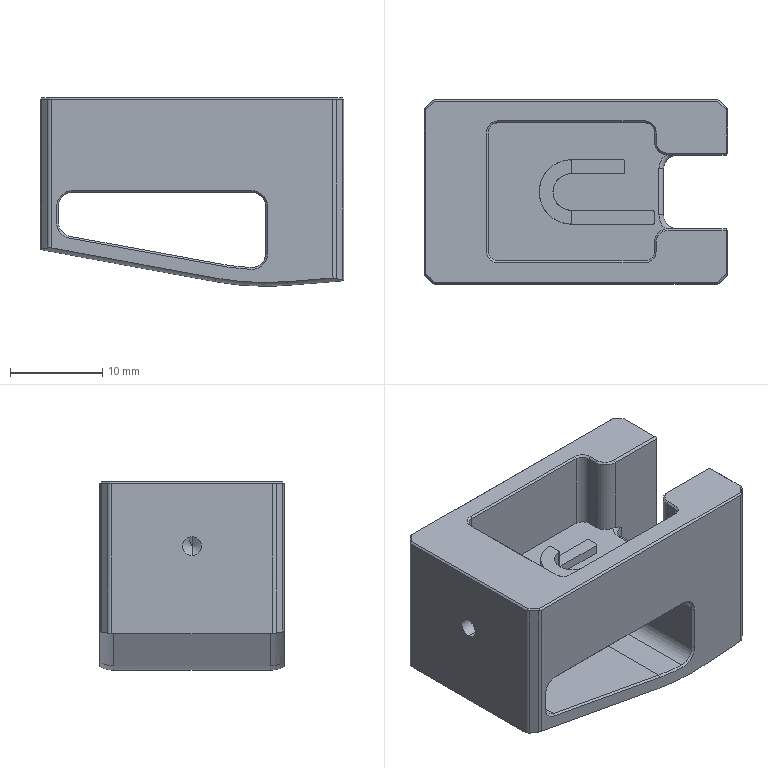NC program | NX | posted with a generic post | part box 33 x 20 x 20.478 mm
Lines 1201 to 2151 of 3438:
(PLANAR_MILL_COPY_1 , TOOL : D3)
N2394 T16 M6
N2396 G54
N2398 G17 G0 G90 X-16.129 Y-4.355 B0. C0. S9500 M3
N2400 G43 Z30. H16
N2402 Z-0.2
N2404 G94 G1 X-16.252 Y-4.41 F1000.
N2406 G3 X-16.838 Y-5.22 R1.
N2408 X-16.939 Y-6.5 R26.5
N2410 G1 X-15.658
N2412 G3 X-14.792 Y-6. R1.
N2414 G1 X-14.734 Y-5.9
N2416 G0 X-16.129 Y-4.355 Z-0.4
N2418 G1 X-16.252 Y-4.41
N2420 G3 X-16.838 Y-5.22 R1.
N2422 X-16.939 Y-6.5 R26.5
N2424 G1 X-15.658
N2426 G3 X-14.792 Y-6. R1.
N2428 G1 X-14.734 Y-5.9
N2430 G0 X-16.129 Y-4.355 Z-0.6
N2432 G1 X-16.252 Y-4.41
N2434 G3 X-16.838 Y-5.22 R1.
N2436 X-16.939 Y-6.5 R26.5
N2438 G1 X-15.658
N2440 G3 X-14.792 Y-6. R1.
N2442 G1 X-14.734 Y-5.9
N2444 G0 X-16.129 Y-4.355 Z-0.8
N2446 G1 X-16.252 Y-4.41
N2448 G3 X-16.838 Y-5.22 R1.
N2450 X-16.939 Y-6.5 R26.5
N2452 G1 X-15.658
N2454 G3 X-14.792 Y-6. R1.
N2456 G1 X-14.734 Y-5.9
N2458 G0 X-16.129 Y-4.355 Z-1.
N2460 G1 X-16.252 Y-4.41
N2462 G3 X-16.838 Y-5.22 R1.
N2464 X-16.939 Y-6.5 R26.5
N2466 G1 X-15.658
N2468 G3 X-14.792 Y-6. R1.
N2470 G1 X-14.734 Y-5.9
N2472 G0 X-16.129 Y-4.355 Z-1.2
N2474 G1 X-16.252 Y-4.41
N2476 G3 X-16.838 Y-5.22 R1.
N2478 X-16.939 Y-6.5 R26.5
N2480 G1 X-15.658
N2482 G3 X-14.792 Y-6. R1.
N2484 G1 X-14.734 Y-5.9
N2486 G0 X-16.129 Y-4.355 Z-1.4
N2488 G1 X-16.252 Y-4.41
N2490 G3 X-16.838 Y-5.22 R1.
N2492 X-16.939 Y-6.5 R26.5
N2494 G1 X-15.658
N2496 G3 X-14.792 Y-6. R1.
N2498 G1 X-14.734 Y-5.9
N2500 G0 X-16.129 Y-4.355 Z-1.6
N2502 G1 X-16.252 Y-4.41
N2504 G3 X-16.838 Y-5.22 R1.
N2506 X-16.939 Y-6.5 R26.5
N2508 G1 X-15.658
N2510 G3 X-14.792 Y-6. R1.
N2512 G1 X-14.734 Y-5.9
N2514 G0 X-16.129 Y-4.355 Z-1.8
N2516 G1 X-16.252 Y-4.41
N2518 G3 X-16.838 Y-5.22 R1.
N2520 X-16.939 Y-6.5 R26.5
N2522 G1 X-15.658
N2524 G3 X-14.792 Y-6. R1.
N2526 G1 X-14.734 Y-5.9
N2528 G0 X-16.129 Y-4.355 Z-2.
N2530 G1 X-16.252 Y-4.41
N2532 G3 X-16.838 Y-5.22 R1.
N2534 X-16.939 Y-6.5 R26.5
N2536 G1 X-15.658
N2538 G3 X-14.792 Y-6. R1.
N2540 G1 X-14.734 Y-5.9
N2542 G0 X-16.129 Y-4.355 Z-2.2
N2544 G1 X-16.252 Y-4.41
N2546 G3 X-16.838 Y-5.22 R1.
N2548 X-16.939 Y-6.5 R26.5
N2550 G1 X-15.658
N2552 G3 X-14.792 Y-6. R1.
N2554 G1 X-14.734 Y-5.9
N2556 G0 X-16.129 Y-4.355 Z-2.4
N2558 G1 X-16.252 Y-4.41
N2560 G3 X-16.838 Y-5.22 R1.
N2562 X-16.939 Y-6.5 R26.5
N2564 G1 X-15.658
N2566 G3 X-14.792 Y-6. R1.
N2568 G1 X-14.734 Y-5.9
N2570 G0 X-16.129 Y-4.355 Z-2.6
N2572 G1 X-16.252 Y-4.41
N2574 G3 X-16.838 Y-5.22 R1.
N2576 X-16.939 Y-6.5 R26.5
N2578 G1 X-15.658
N2580 G3 X-14.792 Y-6. R1.
N2582 G1 X-14.734 Y-5.9
N2584 G0 X-16.129 Y-4.355 Z-2.8
N2586 G1 X-16.252 Y-4.41
N2588 G3 X-16.838 Y-5.22 R1.
N2590 X-16.939 Y-6.5 R26.5
N2592 G1 X-15.658
N2594 G3 X-14.792 Y-6. R1.
N2596 G1 X-14.734 Y-5.9
N2598 G0 X-16.129 Y-4.355 Z-3.
N2600 G1 X-16.252 Y-4.41
N2602 G3 X-16.838 Y-5.22 R1.
N2604 X-16.939 Y-6.5 R26.5
N2606 G1 X-15.658
N2608 G3 X-14.792 Y-6. R1.
N2610 G1 X-14.734 Y-5.9
N2612 G0 X-16.129 Y-4.355 Z-3.2
N2614 G1 X-16.252 Y-4.41
N2616 G3 X-16.838 Y-5.22 R1.
N2618 X-16.939 Y-6.5 R26.5
N2620 G1 X-15.658
N2622 G3 X-14.792 Y-6. R1.
N2624 G1 X-14.734 Y-5.9
N2626 G0 X-16.129 Y-4.355 Z-3.4
N2628 G1 X-16.252 Y-4.41
N2630 G3 X-16.838 Y-5.22 R1.
N2632 X-16.939 Y-6.5 R26.5
N2634 G1 X-15.658
N2636 G3 X-14.792 Y-6. R1.
N2638 G1 X-14.734 Y-5.9
N2640 G0 X-16.129 Y-4.355 Z-3.6
N2642 G1 X-16.252 Y-4.41
N2644 G3 X-16.838 Y-5.22 R1.
N2646 X-16.939 Y-6.5 R26.5
N2648 G1 X-15.658
N2650 G3 X-14.792 Y-6. R1.
N2652 G1 X-14.734 Y-5.9
N2654 G0 X-16.129 Y-4.355 Z-3.8
N2656 G1 X-16.252 Y-4.41
N2658 G3 X-16.838 Y-5.22 R1.
N2660 X-16.939 Y-6.5 R26.5
N2662 G1 X-15.658
N2664 G3 X-14.792 Y-6. R1.
N2666 G1 X-14.734 Y-5.9
N2668 G0 X-16.129 Y-4.355 Z-4.
N2670 G1 X-16.252 Y-4.41
N2672 G3 X-16.838 Y-5.22 R1.
N2674 X-16.939 Y-6.5 R26.5
N2676 G1 X-15.658
N2678 G3 X-14.792 Y-6. R1.
N2680 G1 X-14.734 Y-5.9
N2682 G0 X-16.129 Y-4.355 Z-4.2
N2684 G1 X-16.252 Y-4.41
N2686 G3 X-16.838 Y-5.22 R1.
N2688 X-16.939 Y-6.5 R26.5
N2690 G1 X-15.658
N2692 G3 X-14.792 Y-6. R1.
N2694 G1 X-14.734 Y-5.9
N2696 G0 X-16.129 Y-4.355 Z-4.4
N2698 G1 X-16.252 Y-4.41
N2700 G3 X-16.838 Y-5.22 R1.
N2702 X-16.939 Y-6.5 R26.5
N2704 G1 X-15.658
N2706 G3 X-14.792 Y-6. R1.
N2708 G1 X-14.734 Y-5.9
N2710 G0 X-16.129 Y-4.355 Z-4.6
N2712 G1 X-16.252 Y-4.41
N2714 G3 X-16.838 Y-5.22 R1.
N2716 X-16.939 Y-6.5 R26.5
N2718 G1 X-15.658
N2720 G3 X-14.792 Y-6. R1.
N2722 G1 X-14.734 Y-5.9
N2724 G0 X-16.129 Y-4.355 Z-4.8
N2726 G1 X-16.252 Y-4.41
N2728 G3 X-16.838 Y-5.22 R1.
N2730 X-16.939 Y-6.5 R26.5
N2732 G1 X-15.658
N2734 G3 X-14.792 Y-6. R1.
N2736 G1 X-14.734 Y-5.9
N2738 G0 X-16.129 Y-4.355 Z-5.
N2740 G1 X-16.252 Y-4.41
N2742 G3 X-16.838 Y-5.22 R1.
N2744 X-16.939 Y-6.5 R26.5
N2746 G1 X-15.658
N2748 G3 X-14.792 Y-6. R1.
N2750 G1 X-14.734 Y-5.9
N2752 G0 X-16.129 Y-4.355 Z-5.2
N2754 G1 X-16.252 Y-4.41
N2756 G3 X-16.838 Y-5.22 R1.
N2758 X-16.939 Y-6.5 R26.5
N2760 G1 X-15.658
N2762 G3 X-14.792 Y-6. R1.
N2764 G1 X-14.734 Y-5.9
N2766 G0 X-16.129 Y-4.355 Z-5.4
N2768 G1 X-16.252 Y-4.41
N2770 G3 X-16.838 Y-5.22 R1.
N2772 X-16.939 Y-6.5 R26.5
N2774 G1 X-15.658
N2776 G3 X-14.792 Y-6. R1.
N2778 G1 X-14.734 Y-5.9
N2780 G0 X-16.129 Y-4.355 Z-5.6
N2782 G1 X-16.252 Y-4.41
N2784 G3 X-16.838 Y-5.22 R1.
N2786 X-16.939 Y-6.5 R26.5
N2788 G1 X-15.658
N2790 G3 X-14.792 Y-6. R1.
N2792 G1 X-14.734 Y-5.9
N2794 G0 X-16.129 Y-4.355 Z-5.8
N2796 G1 X-16.252 Y-4.41
N2798 G3 X-16.838 Y-5.22 R1.
N2800 X-16.939 Y-6.5 R26.5
N2802 G1 X-15.658
N2804 G3 X-14.792 Y-6. R1.
N2806 G1 X-14.734 Y-5.9
N2808 G0 X-16.129 Y-4.355 Z-6.
N2810 G1 X-16.252 Y-4.41
N2812 G3 X-16.838 Y-5.22 R1.
N2814 X-16.939 Y-6.5 R26.5
N2816 G1 X-15.658
N2818 G3 X-14.792 Y-6. R1.
N2820 G1 X-14.734 Y-5.9
N2822 G0 X-16.129 Y-4.355 Z-6.2
N2824 G1 X-16.252 Y-4.41
N2826 G3 X-16.838 Y-5.22 R1.
N2828 X-16.939 Y-6.5 R26.5
N2830 G1 X-15.658
N2832 G3 X-14.792 Y-6. R1.
N2834 G1 X-14.734 Y-5.9
N2836 G0 X-16.129 Y-4.355 Z-6.4
N2838 G1 X-16.252 Y-4.41
N2840 G3 X-16.838 Y-5.22 R1.
N2842 X-16.939 Y-6.5 R26.5
N2844 G1 X-15.658
N2846 G3 X-14.792 Y-6. R1.
N2848 G1 X-14.734 Y-5.9
N2850 G0 X-16.129 Y-4.355 Z-6.6
N2852 G1 X-16.252 Y-4.41
N2854 G3 X-16.838 Y-5.22 R1.
N2856 X-16.939 Y-6.5 R26.5
N2858 G1 X-15.658
N2860 G3 X-14.792 Y-6. R1.
N2862 G1 X-14.734 Y-5.9
N2864 G0 X-16.129 Y-4.355 Z-6.8
N2866 G1 X-16.252 Y-4.41
N2868 G3 X-16.838 Y-5.22 R1.
N2870 X-16.939 Y-6.5 R26.5
N2872 G1 X-15.658
N2874 G3 X-14.792 Y-6. R1.
N2876 G1 X-14.734 Y-5.9
N2878 G0 X-16.129 Y-4.355 Z-7.
N2880 G1 X-16.252 Y-4.41
N2882 G3 X-16.838 Y-5.22 R1.
N2884 X-16.939 Y-6.5 R26.5
N2886 G1 X-15.658
N2888 G3 X-14.792 Y-6. R1.
N2890 G1 X-14.734 Y-5.9
N2892 G0 X-16.129 Y-4.355 Z-7.2
N2894 G1 X-16.252 Y-4.41
N2896 G3 X-16.838 Y-5.22 R1.
N2898 X-16.939 Y-6.5 R26.5
N2900 G1 X-15.658
N2902 G3 X-14.792 Y-6. R1.
N2904 G1 X-14.734 Y-5.9
N2906 G0 X-16.129 Y-4.355 Z-7.4
N2908 G1 X-16.252 Y-4.41
N2910 G3 X-16.838 Y-5.22 R1.
N2912 X-16.939 Y-6.5 R26.5
N2914 G1 X-15.658
N2916 G3 X-14.792 Y-6. R1.
N2918 G1 X-14.734 Y-5.9
N2920 G0 X-16.129 Y-4.355 Z-7.6
N2922 G1 X-16.252 Y-4.41
N2924 G3 X-16.838 Y-5.22 R1.
N2926 X-16.939 Y-6.5 R26.5
N2928 G1 X-15.658
N2930 G3 X-14.792 Y-6. R1.
N2932 G1 X-14.734 Y-5.9
N2934 G0 X-16.129 Y-4.355 Z-7.8
N2936 G1 X-16.252 Y-4.41
N2938 G3 X-16.838 Y-5.22 R1.
N2940 X-16.939 Y-6.5 R26.5
N2942 G1 X-15.658
N2944 G3 X-14.792 Y-6. R1.
N2946 G1 X-14.734 Y-5.9
N2948 G0 X-16.129 Y-4.355 Z-8.
N2950 G1 X-16.252 Y-4.41
N2952 G3 X-16.838 Y-5.22 R1.
N2954 X-16.939 Y-6.5 R26.5
N2956 G1 X-15.658
N2958 G3 X-14.792 Y-6. R1.
N2960 G1 X-14.734 Y-5.9
N2962 G0 X-16.129 Y-4.355 Z-8.2
N2964 G1 X-16.252 Y-4.41
N2966 G3 X-16.838 Y-5.22 R1.
N2968 X-16.939 Y-6.5 R26.5
N2970 G1 X-15.658
N2972 G3 X-14.792 Y-6. R1.
N2974 G1 X-14.734 Y-5.9
N2976 G0 X-16.129 Y-4.355 Z-8.4
N2978 G1 X-16.252 Y-4.41
N2980 G3 X-16.838 Y-5.22 R1.
N2982 X-16.939 Y-6.5 R26.5
N2984 G1 X-15.658
N2986 G3 X-14.792 Y-6. R1.
N2988 G1 X-14.734 Y-5.9
N2990 G0 X-16.129 Y-4.355 Z-8.6
N2992 G1 X-16.252 Y-4.41
N2994 G3 X-16.838 Y-5.22 R1.
N2996 X-16.939 Y-6.5 R26.5
N2998 G1 X-15.658
N3000 G3 X-14.792 Y-6. R1.
N3002 G1 X-14.734 Y-5.9
N3004 G0 X-16.129 Y-4.355 Z-8.8
N3006 G1 X-16.252 Y-4.41
N3008 G3 X-16.838 Y-5.22 R1.
N3010 X-16.939 Y-6.5 R26.5
N3012 G1 X-15.658
N3014 G3 X-14.792 Y-6. R1.
N3016 G1 X-14.734 Y-5.9
N3018 G0 X-16.129 Y-4.355 Z-9.
N3020 G1 X-16.252 Y-4.41
N3022 G3 X-16.838 Y-5.22 R1.
N3024 X-16.939 Y-6.5 R26.5
N3026 G1 X-15.658
N3028 G3 X-14.792 Y-6. R1.
N3030 G1 X-14.734 Y-5.9
N3032 G0 X-16.129 Y-4.355 Z-9.2
N3034 G1 X-16.252 Y-4.41
N3036 G3 X-16.838 Y-5.22 R1.
N3038 X-16.939 Y-6.5 R26.5
N3040 G1 X-15.658
N3042 G3 X-14.792 Y-6. R1.
N3044 G1 X-14.734 Y-5.9
N3046 G0 X-16.129 Y-4.355 Z-9.4
N3048 G1 X-16.252 Y-4.41
N3050 G3 X-16.838 Y-5.22 R1.
N3052 X-16.939 Y-6.5 R26.5
N3054 G1 X-15.658
N3056 G3 X-14.792 Y-6. R1.
N3058 G1 X-14.734 Y-5.9
N3060 G0 X-16.129 Y-4.355 Z-9.6
N3062 G1 X-16.252 Y-4.41
N3064 G3 X-16.838 Y-5.22 R1.
N3066 X-16.939 Y-6.5 R26.5
N3068 G1 X-15.658
N3070 G3 X-14.792 Y-6. R1.
N3072 G1 X-14.734 Y-5.9
N3074 G0 X-16.129 Y-4.355 Z-9.8
N3076 G1 X-16.252 Y-4.41
N3078 G3 X-16.838 Y-5.22 R1.
N3080 X-16.939 Y-6.5 R26.5
N3082 G1 X-15.658
N3084 G3 X-14.792 Y-6. R1.
N3086 G1 X-14.734 Y-5.9
N3088 G0 X-16.129 Y-4.355 Z-10.
N3090 G1 X-16.252 Y-4.41
N3092 G3 X-16.838 Y-5.22 R1.
N3094 X-16.939 Y-6.5 R26.5
N3096 G1 X-15.658
N3098 G3 X-14.792 Y-6. R1.
N3100 G1 X-14.734 Y-5.9
N3102 G0 X-16.129 Y-4.355 Z-10.2
N3104 G1 X-16.252 Y-4.41
N3106 G3 X-16.838 Y-5.22 R1.
N3108 X-16.939 Y-6.5 R26.5
N3110 G1 X-15.658
N3112 G3 X-14.792 Y-6. R1.
N3114 G1 X-14.734 Y-5.9
N3116 G0 X-16.129 Y-4.355 Z-10.4
N3118 G1 X-16.252 Y-4.41
N3120 G3 X-16.838 Y-5.22 R1.
N3122 X-16.939 Y-6.5 R26.5
N3124 G1 X-15.658
N3126 G3 X-14.792 Y-6. R1.
N3128 G1 X-14.734 Y-5.9
N3130 G0 X-16.129 Y-4.355 Z-10.6
N3132 G1 X-16.252 Y-4.41
N3134 G3 X-16.838 Y-5.22 R1.
N3136 X-16.939 Y-6.5 R26.5
N3138 G1 X-15.658
N3140 G3 X-14.792 Y-6. R1.
N3142 G1 X-14.734 Y-5.9
N3144 G0 X-16.129 Y-4.355 Z-10.8
N3146 G1 X-16.252 Y-4.41
N3148 G3 X-16.838 Y-5.22 R1.
N3150 X-16.939 Y-6.5 R26.5
N3152 G1 X-15.658
N3154 G3 X-14.792 Y-6. R1.
N3156 G1 X-14.734 Y-5.9
N3158 G0 X-16.129 Y-4.355 Z-11.
N3160 G1 X-16.252 Y-4.41
N3162 G3 X-16.838 Y-5.22 R1.
N3164 X-16.939 Y-6.5 R26.5
N3166 G1 X-15.658
N3168 G3 X-14.792 Y-6. R1.
N3170 G1 X-14.734 Y-5.9
N3172 G0 X-16.129 Y-4.355 Z-11.2
N3174 G1 X-16.252 Y-4.41
N3176 G3 X-16.838 Y-5.22 R1.
N3178 X-16.939 Y-6.5 R26.5
N3180 G1 X-15.658
N3182 G3 X-14.792 Y-6. R1.
N3184 G1 X-14.734 Y-5.9
N3186 G0 X-16.129 Y-4.355 Z-11.4
N3188 G1 X-16.252 Y-4.41
N3190 G3 X-16.838 Y-5.22 R1.
N3192 X-16.939 Y-6.5 R26.5
N3194 G1 X-15.658
N3196 G3 X-14.792 Y-6. R1.
N3198 G1 X-14.734 Y-5.9
N3200 G0 X-16.129 Y-4.355 Z-11.6
N3202 G1 X-16.252 Y-4.41
N3204 G3 X-16.838 Y-5.22 R1.
N3206 X-16.939 Y-6.5 R26.5
N3208 G1 X-15.658
N3210 G3 X-14.792 Y-6. R1.
N3212 G1 X-14.734 Y-5.9
N3214 G0 X-16.129 Y-4.355 Z-11.8
N3216 G1 X-16.252 Y-4.41
N3218 G3 X-16.838 Y-5.22 R1.
N3220 X-16.939 Y-6.5 R26.5
N3222 G1 X-15.658
N3224 G3 X-14.792 Y-6. R1.
N3226 G1 X-14.734 Y-5.9
N3228 G0 X-16.129 Y-4.355 Z-12.
N3230 G1 X-16.252 Y-4.41
N3232 G3 X-16.838 Y-5.22 R1.
N3234 X-16.939 Y-6.5 R26.5
N3236 G1 X-15.658
N3238 G3 X-14.792 Y-6. R1.
N3240 G1 X-14.734 Y-5.9
N3242 G0 X-16.129 Y-4.355 Z-12.2
N3244 G1 X-16.252 Y-4.41
N3246 G3 X-16.838 Y-5.22 R1.
N3248 X-16.939 Y-6.5 R26.5
N3250 G1 X-15.658
N3252 G3 X-14.792 Y-6. R1.
N3254 G1 X-14.734 Y-5.9
N3256 G0 X-16.129 Y-4.355 Z-12.4
N3258 G1 X-16.252 Y-4.41
N3260 G3 X-16.838 Y-5.22 R1.
N3262 X-16.939 Y-6.5 R26.5
N3264 G1 X-15.658
N3266 G3 X-14.792 Y-6. R1.
N3268 G1 X-14.734 Y-5.9
N3270 G0 X-16.129 Y-4.355 Z-12.6
N3272 G1 X-16.252 Y-4.41
N3274 G3 X-16.838 Y-5.22 R1.
N3276 X-16.939 Y-6.5 R26.5
N3278 G1 X-15.658
N3280 G3 X-14.792 Y-6. R1.
N3282 G1 X-14.734 Y-5.9
N3284 G0 X-16.129 Y-4.355 Z-12.8
N3286 G1 X-16.252 Y-4.41
N3288 G3 X-16.838 Y-5.22 R1.
N3290 X-16.939 Y-6.5 R26.5
N3292 G1 X-15.658
N3294 G3 X-14.792 Y-6. R1.
N3296 G1 X-14.734 Y-5.9
N3298 G0 X-16.129 Y-4.355 Z-13.
N3300 G1 X-16.252 Y-4.41
N3302 G3 X-16.838 Y-5.22 R1.
N3304 X-16.939 Y-6.5 R26.5
N3306 G1 X-15.658
N3308 G3 X-14.792 Y-6. R1.
N3310 G1 X-14.734 Y-5.9
N3312 G0 X-16.129 Y-4.355 Z-13.2
N3314 G1 X-16.252 Y-4.41
N3316 G3 X-16.838 Y-5.22 R1.
N3318 X-16.939 Y-6.5 R26.5
N3320 G1 X-15.658
N3322 G3 X-14.792 Y-6. R1.
N3324 G1 X-14.734 Y-5.9
N3326 G0 X-16.129 Y-4.355 Z-13.4
N3328 G1 X-16.252 Y-4.41
N3330 G3 X-16.838 Y-5.22 R1.
N3332 X-16.939 Y-6.5 R26.5
N3334 G1 X-15.658
N3336 G3 X-14.792 Y-6. R1.
N3338 G1 X-14.734 Y-5.9
N3340 G0 X-16.129 Y-4.355 Z-13.6
N3342 G1 X-16.252 Y-4.41
N3344 G3 X-16.838 Y-5.22 R1.
N3346 X-16.939 Y-6.5 R26.5
N3348 G1 X-15.658
N3350 G3 X-14.792 Y-6. R1.
N3352 G1 X-14.734 Y-5.9
N3354 G0 X-16.129 Y-4.355 Z-13.8
N3356 G1 X-16.252 Y-4.41
N3358 G3 X-16.838 Y-5.22 R1.
N3360 X-16.939 Y-6.5 R26.5
N3362 G1 X-15.658
N3364 G3 X-14.792 Y-6. R1.
N3366 G1 X-14.734 Y-5.9
N3368 G0 X-16.129 Y-4.355 Z-14.
N3370 G1 X-16.252 Y-4.41
N3372 G3 X-16.838 Y-5.22 R1.
N3374 X-16.939 Y-6.5 R26.5
N3376 G1 X-15.658
N3378 G3 X-14.792 Y-6. R1.
N3380 G1 X-14.734 Y-5.9
N3382 G0 X-16.129 Y-4.355 Z-14.2
N3384 G1 X-16.252 Y-4.41
N3386 G3 X-16.838 Y-5.22 R1.
N3388 X-16.939 Y-6.5 R26.5
N3390 G1 X-15.658
N3392 G3 X-14.792 Y-6. R1.
N3394 G1 X-14.734 Y-5.9
N3396 G0 X-16.129 Y-4.355 Z-14.4
N3398 G1 X-16.252 Y-4.41
N3400 G3 X-16.838 Y-5.22 R1.
N3402 X-16.939 Y-6.5 R26.5
N3404 G1 X-15.658
N3406 G3 X-14.792 Y-6. R1.
N3408 G1 X-14.734 Y-5.9
N3410 G0 X-16.129 Y-4.355 Z-14.6
N3412 G1 X-16.252 Y-4.41
N3414 G3 X-16.838 Y-5.22 R1.
N3416 X-16.939 Y-6.5 R26.5
N3418 G1 X-15.658
N3420 G3 X-14.792 Y-6. R1.
N3422 G1 X-14.734 Y-5.9
N3424 G0 X-16.129 Y-4.355 Z-14.8
N3426 G1 X-16.252 Y-4.41
N3428 G3 X-16.838 Y-5.22 R1.
N3430 X-16.939 Y-6.5 R26.5
N3432 G1 X-15.658
N3434 G3 X-14.792 Y-6. R1.
N3436 G1 X-14.734 Y-5.9
N3438 G0 X-16.129 Y-4.355 Z-15.
N3440 G1 X-16.252 Y-4.41
N3442 G3 X-16.838 Y-5.22 R1.
N3444 X-16.939 Y-6.5 R26.5
N3446 G1 X-15.658
N3448 G3 X-14.792 Y-6. R1.
N3450 G1 X-14.734 Y-5.9
N3452 G0 X-16.129 Y-4.355 Z-15.2
N3454 G1 X-16.252 Y-4.41
N3456 G3 X-16.838 Y-5.22 R1.
N3458 X-16.939 Y-6.5 R26.5
N3460 G1 X-15.658
N3462 G3 X-14.792 Y-6. R1.
N3464 G1 X-14.734 Y-5.9
N3466 G0 X-16.129 Y-4.355 Z-15.4
N3468 G1 X-16.252 Y-4.41
N3470 G3 X-16.838 Y-5.22 R1.
N3472 X-16.939 Y-6.5 R26.5
N3474 G1 X-15.658
N3476 G3 X-14.792 Y-6. R1.
N3478 G1 X-14.734 Y-5.9
N3480 G0 X-16.129 Y-4.355 Z-15.6
N3482 G1 X-16.252 Y-4.41
N3484 G3 X-16.838 Y-5.22 R1.
N3486 X-16.939 Y-6.5 R26.5
N3488 G1 X-15.658
N3490 G3 X-14.792 Y-6. R1.
N3492 G1 X-14.734 Y-5.9
N3494 G0 X-16.129 Y-4.355 Z-15.8
N3496 G1 X-16.252 Y-4.41
N3498 G3 X-16.838 Y-5.22 R1.
N3500 X-16.939 Y-6.5 R26.5
N3502 G1 X-15.658
N3504 G3 X-14.792 Y-6. R1.
N3506 G1 X-14.734 Y-5.9
N3508 G0 X-16.129 Y-4.355 Z-16.
N3510 G1 X-16.252 Y-4.41
N3512 G3 X-16.838 Y-5.22 R1.
N3514 X-16.939 Y-6.5 R26.5
N3516 G1 X-15.658
N3518 G3 X-14.792 Y-6. R1.
N3520 G1 X-14.734 Y-5.9
N3522 G0 X-16.129 Y-4.355 Z-16.2
N3524 G1 X-16.252 Y-4.41
N3526 G3 X-16.838 Y-5.22 R1.
N3528 X-16.939 Y-6.5 R26.5
N3530 G1 X-15.658
N3532 G3 X-14.792 Y-6. R1.
N3534 G1 X-14.734 Y-5.9
N3536 G0 X-16.129 Y-4.355 Z-16.4
N3538 G1 X-16.252 Y-4.41
N3540 G3 X-16.838 Y-5.22 R1.
N3542 X-16.939 Y-6.5 R26.5
N3544 G1 X-15.658
N3546 G3 X-14.792 Y-6. R1.
N3548 G1 X-14.734 Y-5.9
N3550 G0 X-16.129 Y-4.355 Z-16.6
N3552 G1 X-16.252 Y-4.41
N3554 G3 X-16.838 Y-5.22 R1.
N3556 X-16.939 Y-6.5 R26.5
N3558 G1 X-15.658
N3560 G3 X-14.792 Y-6. R1.
N3562 G1 X-14.734 Y-5.9
N3564 G0 X-16.129 Y-4.355 Z-16.8
N3566 G1 X-16.252 Y-4.41
N3568 G3 X-16.838 Y-5.22 R1.
N3570 X-16.939 Y-6.5 R26.5
N3572 G1 X-15.658
N3574 G3 X-14.792 Y-6. R1.
N3576 G1 X-14.734 Y-5.9
N3578 G0 X-16.129 Y-4.355 Z-17.
N3580 G1 X-16.252 Y-4.41
N3582 G3 X-16.838 Y-5.22 R1.
N3584 X-16.939 Y-6.5 R26.5
N3586 G1 X-15.658
N3588 G3 X-14.792 Y-6. R1.
N3590 G1 X-14.734 Y-5.9
N3592 G0 X-16.129 Y-4.355 Z-17.2
N3594 G1 X-16.252 Y-4.41
N3596 G3 X-16.838 Y-5.22 R1.
N3598 X-16.939 Y-6.5 R26.5
N3600 G1 X-15.658
N3602 G3 X-14.792 Y-6. R1.
N3604 G1 X-14.734 Y-5.9
N3606 G0 X-16.129 Y-4.355 Z-17.4
N3608 G1 X-16.252 Y-4.41
N3610 G3 X-16.838 Y-5.22 R1.
N3612 X-16.939 Y-6.5 R26.5
N3614 G1 X-15.658
N3616 G3 X-14.792 Y-6. R1.
N3618 G1 X-14.734 Y-5.9
N3620 G0 X-16.129 Y-4.355 Z-17.6
N3622 G1 X-16.252 Y-4.41
N3624 G3 X-16.838 Y-5.22 R1.
N3626 X-16.939 Y-6.5 R26.5
N3628 G1 X-15.658
N3630 G3 X-14.792 Y-6. R1.
N3632 G1 X-14.734 Y-5.9
N3634 G0 X-16.129 Y-4.355 Z-17.8
N3636 G1 X-16.252 Y-4.41
N3638 G3 X-16.838 Y-5.22 R1.
N3640 X-16.939 Y-6.5 R26.5
N3642 G1 X-15.658
N3644 G3 X-14.792 Y-6. R1.
N3646 G1 X-14.734 Y-5.9
N3648 G0 X-16.129 Y-4.355 Z-18.
N3650 G1 X-16.252 Y-4.41
N3652 G3 X-16.838 Y-5.22 R1.
N3654 X-16.939 Y-6.5 R26.5
N3656 G1 X-15.658
N3658 G3 X-14.792 Y-6. R1.
N3660 G1 X-14.734 Y-5.9
N3662 G0 X-16.129 Y-4.355 Z-18.2
N3664 G1 X-16.252 Y-4.41
N3666 G3 X-16.838 Y-5.22 R1.
N3668 X-16.939 Y-6.5 R26.5
N3670 G1 X-15.658
N3672 G3 X-14.792 Y-6. R1.
N3674 G1 X-14.734 Y-5.9
N3676 G0 X-16.129 Y-4.355 Z-18.4
N3678 G1 X-16.252 Y-4.41
N3680 G3 X-16.838 Y-5.22 R1.
N3682 X-16.939 Y-6.5 R26.5
N3684 G1 X-15.658
N3686 G3 X-14.792 Y-6. R1.
N3688 G1 X-14.734 Y-5.9
N3690 G0 X-16.129 Y-4.355 Z-18.6
N3692 G1 X-16.252 Y-4.41
N3694 G3 X-16.838 Y-5.22 R1.
N3696 X-16.939 Y-6.5 R26.5
N3698 G1 X-15.658
N3700 G3 X-14.792 Y-6. R1.
N3702 G1 X-14.734 Y-5.9
N3704 G0 X-16.129 Y-4.355 Z-18.8
N3706 G1 X-16.252 Y-4.41
N3708 G3 X-16.838 Y-5.22 R1.
N3710 X-16.939 Y-6.5 R26.5
N3712 G1 X-15.658
N3714 G3 X-14.792 Y-6. R1.
N3716 G1 X-14.734 Y-5.9
N3718 G0 X-16.129 Y-4.355 Z-19.
N3720 G1 X-16.252 Y-4.41
N3722 G3 X-16.838 Y-5.22 R1.
N3724 X-16.939 Y-6.5 R26.5
N3726 G1 X-15.658
N3728 G3 X-14.792 Y-6. R1.
N3730 G1 X-14.734 Y-5.9
N3732 G0 X-16.129 Y-4.355 Z-19.2
N3734 G1 X-16.252 Y-4.41
N3736 G3 X-16.838 Y-5.22 R1.
N3738 X-16.939 Y-6.5 R26.5
N3740 G1 X-15.658
N3742 G3 X-14.792 Y-6. R1.
N3744 G1 X-14.734 Y-5.9
N3746 G0 X-16.129 Y-4.355 Z-19.4
N3748 G1 X-16.252 Y-4.41
N3750 G3 X-16.838 Y-5.22 R1.
N3752 X-16.939 Y-6.5 R26.5
N3754 G1 X-15.658
N3756 G3 X-14.792 Y-6. R1.
N3758 G1 X-14.734 Y-5.9
N3760 G0 X-16.129 Y-4.355 Z-19.6
N3762 G1 X-16.252 Y-4.41
N3764 G3 X-16.838 Y-5.22 R1.
N3766 X-16.939 Y-6.5 R26.5
N3768 G1 X-15.658
N3770 G3 X-14.792 Y-6. R1.
N3772 G1 X-14.734 Y-5.9
N3774 G0 X-16.129 Y-4.355 Z-19.8
N3776 G1 X-16.252 Y-4.41
N3778 G3 X-16.838 Y-5.22 R1.
N3780 X-16.939 Y-6.5 R26.5
N3782 G1 X-15.658
N3784 G3 X-14.792 Y-6. R1.
N3786 G1 X-14.734 Y-5.9
N3788 G0 X-16.129 Y-4.355 Z-20.
N3790 G1 X-16.252 Y-4.41
N3792 G3 X-16.838 Y-5.22 R1.
N3794 X-16.939 Y-6.5 R26.5
N3796 G1 X-15.658
N3798 G3 X-14.792 Y-6. R1.
N3800 G1 X-14.734 Y-5.9
N3802 G0 Z30.
N3804 X-13.972
N3806 Z-0.2
N3808 G1 X-13.914 Y-6.
N3810 G3 X-13.048 Y-6.5 R1.
N3812 G1 X-11.8
N3814 Y-5.252
N3816 G3 X-12.3 Y-4.386 R1.
N3818 G1 X-12.4 Y-4.328
N3820 G0 X-13.972 Y-5.9 Z-0.4
N3822 G1 X-13.914 Y-6.
N3824 G3 X-13.048 Y-6.5 R1.
N3826 G1 X-11.8
N3828 Y-5.252
N3830 G3 X-12.3 Y-4.386 R1.
N3832 G1 X-12.4 Y-4.328
N3834 G0 X-13.972 Y-5.9 Z-0.6
N3836 G1 X-13.914 Y-6.
N3838 G3 X-13.048 Y-6.5 R1.
N3840 G1 X-11.8
N3842 Y-5.252
N3844 G3 X-12.3 Y-4.386 R1.
N3846 G1 X-12.4 Y-4.328
N3848 G0 X-13.972 Y-5.9 Z-0.8
N3850 G1 X-13.914 Y-6.
N3852 G3 X-13.048 Y-6.5 R1.
N3854 G1 X-11.8
N3856 Y-5.252
N3858 G3 X-12.3 Y-4.386 R1.
N3860 G1 X-12.4 Y-4.328
N3862 G0 X-13.972 Y-5.9 Z-1.
N3864 G1 X-13.914 Y-6.
N3866 G3 X-13.048 Y-6.5 R1.
N3868 G1 X-11.8
N3870 Y-5.252
N3872 G3 X-12.3 Y-4.386 R1.
N3874 G1 X-12.4 Y-4.328
N3876 G0 X-13.972 Y-5.9 Z-1.2
N3878 G1 X-13.914 Y-6.
N3880 G3 X-13.048 Y-6.5 R1.
N3882 G1 X-11.8
N3884 Y-5.252
N3886 G3 X-12.3 Y-4.386 R1.
N3888 G1 X-12.4 Y-4.328
N3890 G0 X-13.972 Y-5.9 Z-1.4
N3892 G1 X-13.914 Y-6.
N3894 G3 X-13.048 Y-6.5 R1.
N3896 G1 X-11.8
N3898 Y-5.252
N3900 G3 X-12.3 Y-4.386 R1.
N3902 G1 X-12.4 Y-4.328
N3904 G0 X-13.972 Y-5.9 Z-1.6
N3906 G1 X-13.914 Y-6.
N3908 G3 X-13.048 Y-6.5 R1.
N3910 G1 X-11.8
N3912 Y-5.252
N3914 G3 X-12.3 Y-4.386 R1.
N3916 G1 X-12.4 Y-4.328
N3918 G0 X-13.972 Y-5.9 Z-1.8
N3920 G1 X-13.914 Y-6.
N3922 G3 X-13.048 Y-6.5 R1.
N3924 G1 X-11.8
N3926 Y-5.252
N3928 G3 X-12.3 Y-4.386 R1.
N3930 G1 X-12.4 Y-4.328
N3932 G0 X-13.972 Y-5.9 Z-2.
N3934 G1 X-13.914 Y-6.
N3936 G3 X-13.048 Y-6.5 R1.
N3938 G1 X-11.8
N3940 Y-5.252
N3942 G3 X-12.3 Y-4.386 R1.
N3944 G1 X-12.4 Y-4.328
N3946 G0 X-13.972 Y-5.9 Z-2.2
N3948 G1 X-13.914 Y-6.
N3950 G3 X-13.048 Y-6.5 R1.
N3952 G1 X-11.8
N3954 Y-5.252
N3956 G3 X-12.3 Y-4.386 R1.
N3958 G1 X-12.4 Y-4.328
N3960 G0 X-13.972 Y-5.9 Z-2.4
N3962 G1 X-13.914 Y-6.
N3964 G3 X-13.048 Y-6.5 R1.
N3966 G1 X-11.8
N3968 Y-5.252
N3970 G3 X-12.3 Y-4.386 R1.
N3972 G1 X-12.4 Y-4.328
N3974 G0 X-13.972 Y-5.9 Z-2.6
N3976 G1 X-13.914 Y-6.
N3978 G3 X-13.048 Y-6.5 R1.
N3980 G1 X-11.8
N3982 Y-5.252
N3984 G3 X-12.3 Y-4.386 R1.
N3986 G1 X-12.4 Y-4.328
N3988 G0 X-13.972 Y-5.9 Z-2.8
N3990 G1 X-13.914 Y-6.
N3992 G3 X-13.048 Y-6.5 R1.
N3994 G1 X-11.8
N3996 Y-5.252
N3998 G3 X-12.3 Y-4.386 R1.
N4000 G1 X-12.4 Y-4.328
N4002 G0 X-13.972 Y-5.9 Z-3.
N4004 G1 X-13.914 Y-6.
N4006 G3 X-13.048 Y-6.5 R1.
N4008 G1 X-11.8
N4010 Y-5.252
N4012 G3 X-12.3 Y-4.386 R1.
N4014 G1 X-12.4 Y-4.328
N4016 G0 X-13.972 Y-5.9 Z-3.2
N4018 G1 X-13.914 Y-6.
N4020 G3 X-13.048 Y-6.5 R1.
N4022 G1 X-11.8
N4024 Y-5.252
N4026 G3 X-12.3 Y-4.386 R1.
N4028 G1 X-12.4 Y-4.328
N4030 G0 X-13.972 Y-5.9 Z-3.4
N4032 G1 X-13.914 Y-6.
N4034 G3 X-13.048 Y-6.5 R1.
N4036 G1 X-11.8
N4038 Y-5.252
N4040 G3 X-12.3 Y-4.386 R1.
N4042 G1 X-12.4 Y-4.328
N4044 G0 X-13.972 Y-5.9 Z-3.6
N4046 G1 X-13.914 Y-6.
N4048 G3 X-13.048 Y-6.5 R1.
N4050 G1 X-11.8
N4052 Y-5.252
N4054 G3 X-12.3 Y-4.386 R1.
N4056 G1 X-12.4 Y-4.328
N4058 G0 X-13.972 Y-5.9 Z-3.8
N4060 G1 X-13.914 Y-6.
N4062 G3 X-13.048 Y-6.5 R1.
N4064 G1 X-11.8
N4066 Y-5.252
N4068 G3 X-12.3 Y-4.386 R1.
N4070 G1 X-12.4 Y-4.328
N4072 G0 X-13.972 Y-5.9 Z-4.
N4074 G1 X-13.914 Y-6.
N4076 G3 X-13.048 Y-6.5 R1.
N4078 G1 X-11.8
N4080 Y-5.252
N4082 G3 X-12.3 Y-4.386 R1.
N4084 G1 X-12.4 Y-4.328
N4086 G0 X-13.972 Y-5.9 Z-4.2
N4088 G1 X-13.914 Y-6.
N4090 G3 X-13.048 Y-6.5 R1.
N4092 G1 X-11.8
N4094 Y-5.252
N4096 G3 X-12.3 Y-4.386 R1.
N4098 G1 X-12.4 Y-4.328
N4100 G0 X-13.972 Y-5.9 Z-4.4
N4102 G1 X-13.914 Y-6.
N4104 G3 X-13.048 Y-6.5 R1.
N4106 G1 X-11.8
N4108 Y-5.252
N4110 G3 X-12.3 Y-4.386 R1.
N4112 G1 X-12.4 Y-4.328
N4114 G0 X-13.972 Y-5.9 Z-4.6
N4116 G1 X-13.914 Y-6.
N4118 G3 X-13.048 Y-6.5 R1.
N4120 G1 X-11.8
N4122 Y-5.252
N4124 G3 X-12.3 Y-4.386 R1.
N4126 G1 X-12.4 Y-4.328
N4128 G0 X-13.972 Y-5.9 Z-4.8
N4130 G1 X-13.914 Y-6.
N4132 G3 X-13.048 Y-6.5 R1.
N4134 G1 X-11.8
N4136 Y-5.252
N4138 G3 X-12.3 Y-4.386 R1.
N4140 G1 X-12.4 Y-4.328
N4142 G0 X-13.972 Y-5.9 Z-5.
N4144 G1 X-13.914 Y-6.
N4146 G3 X-13.048 Y-6.5 R1.
N4148 G1 X-11.8
N4150 Y-5.252
N4152 G3 X-12.3 Y-4.386 R1.
N4154 G1 X-12.4 Y-4.328
N4156 G0 X-13.972 Y-5.9 Z-5.2
N4158 G1 X-13.914 Y-6.
N4160 G3 X-13.048 Y-6.5 R1.
N4162 G1 X-11.8
N4164 Y-5.252
N4166 G3 X-12.3 Y-4.386 R1.
N4168 G1 X-12.4 Y-4.328
N4170 G0 X-13.972 Y-5.9 Z-5.4
N4172 G1 X-13.914 Y-6.
N4174 G3 X-13.048 Y-6.5 R1.
N4176 G1 X-11.8
N4178 Y-5.252
N4180 G3 X-12.3 Y-4.386 R1.
N4182 G1 X-12.4 Y-4.328
N4184 G0 X-13.972 Y-5.9 Z-5.6
N4186 G1 X-13.914 Y-6.
N4188 G3 X-13.048 Y-6.5 R1.
N4190 G1 X-11.8
N4192 Y-5.252
N4194 G3 X-12.3 Y-4.386 R1.
N4196 G1 X-12.4 Y-4.328
N4198 G0 X-13.972 Y-5.9 Z-5.8
N4200 G1 X-13.914 Y-6.
N4202 G3 X-13.048 Y-6.5 R1.
N4204 G1 X-11.8
N4206 Y-5.252
N4208 G3 X-12.3 Y-4.386 R1.
N4210 G1 X-12.4 Y-4.328
N4212 G0 X-13.972 Y-5.9 Z-6.
N4214 G1 X-13.914 Y-6.
N4216 G3 X-13.048 Y-6.5 R1.
N4218 G1 X-11.8
N4220 Y-5.252
N4222 G3 X-12.3 Y-4.386 R1.
N4224 G1 X-12.4 Y-4.328
N4226 G0 X-13.972 Y-5.9 Z-6.2
N4228 G1 X-13.914 Y-6.
N4230 G3 X-13.048 Y-6.5 R1.
N4232 G1 X-11.8
N4234 Y-5.252
N4236 G3 X-12.3 Y-4.386 R1.
N4238 G1 X-12.4 Y-4.328
N4240 G0 X-13.972 Y-5.9 Z-6.4
N4242 G1 X-13.914 Y-6.
N4244 G3 X-13.048 Y-6.5 R1.
N4246 G1 X-11.8
N4248 Y-5.252
N4250 G3 X-12.3 Y-4.386 R1.
N4252 G1 X-12.4 Y-4.328
N4254 G0 X-13.972 Y-5.9 Z-6.6
N4256 G1 X-13.914 Y-6.
N4258 G3 X-13.048 Y-6.5 R1.
N4260 G1 X-11.8
N4262 Y-5.252
N4264 G3 X-12.3 Y-4.386 R1.
N4266 G1 X-12.4 Y-4.328
N4268 G0 X-13.972 Y-5.9 Z-6.8
N4270 G1 X-13.914 Y-6.
N4272 G3 X-13.048 Y-6.5 R1.
N4274 G1 X-11.8
N4276 Y-5.252
N4278 G3 X-12.3 Y-4.386 R1.
N4280 G1 X-12.4 Y-4.328
N4282 G0 X-13.972 Y-5.9 Z-7.
N4284 G1 X-13.914 Y-6.
N4286 G3 X-13.048 Y-6.5 R1.
N4288 G1 X-11.8